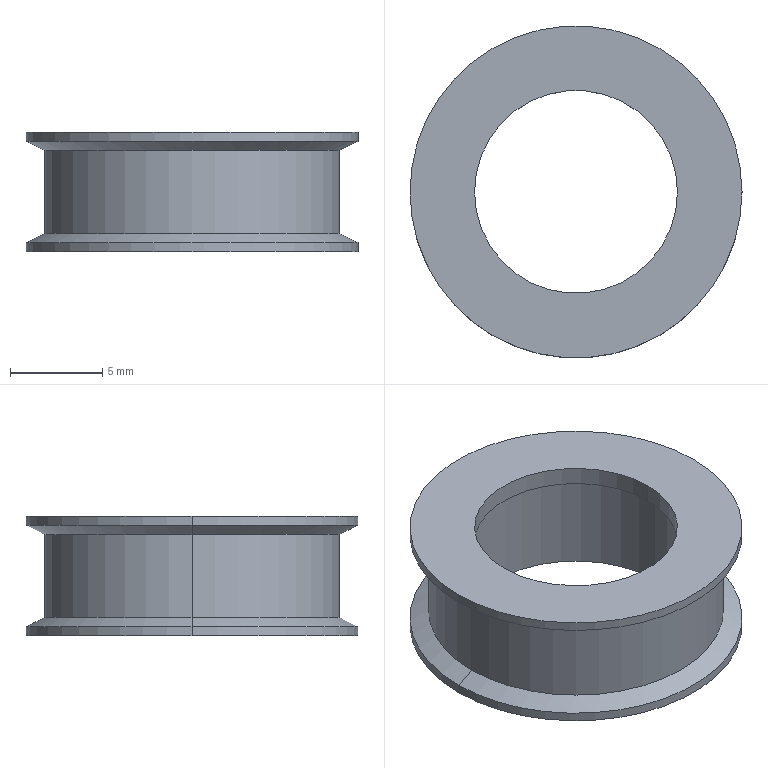Part | STEP file | 602-08-0005 | 1 solid | 17 faces | box 18 x 18 x 6.5 mm | volume 669.421 mm3 | cylinder 10 | cone 4 | plane 3 | commonest cylinder face diameters 18 x4 11 x2 12 x2 16 x2
STEP:
#1=CARTESIAN_POINT('',(0.,0.,0.));
#2=DIRECTION('',(0.,0.,1.));
#3=DIRECTION('',(1.,0.,0.));
#4=AXIS2_PLACEMENT_3D('',#1,#2,#3);
#5=CARTESIAN_POINT('',(-6.,0.,5.5));
#6=VERTEX_POINT('',#5);
#7=CARTESIAN_POINT('',(-6.,0.,0.));
#8=VERTEX_POINT('',#7);
#9=CARTESIAN_POINT('',(-6.,0.,5.5));
#10=DIRECTION('',(0.,0.,-1.));
#11=VECTOR('',#10,1.);
#12=LINE('',#9,#11);
#13=CARTESIAN_POINT('',(0.,0.,5.5));
#14=DIRECTION('',(0.,0.,-1.));
#15=DIRECTION('',(-1.,0.,0.));
#16=AXIS2_PLACEMENT_3D('',#13,#14,#15);
#17=CYLINDRICAL_SURFACE('',#16,6.);
#18=CARTESIAN_POINT('',(6.283,0.));
#19=DIRECTION('',(0.,1.));
#20=VECTOR('',#19,1.);
#21=LINE('',#18,#20);
#22=(GEOMETRIC_REPRESENTATION_CONTEXT(2)PARAMETRIC_REPRESENTATION_CONTEXT()REPRESENTATION_CONTEXT('',''));
#23=DEFINITIONAL_REPRESENTATION('',(#21),#22);
#24=PCURVE('',#17,#23);
#25=CARTESIAN_POINT('',(0.,0.,5.5));
#26=DIRECTION('',(0.,0.,-1.));
#27=DIRECTION('',(-1.,0.,0.));
#28=AXIS2_PLACEMENT_3D('',#25,#26,#27);
#29=CYLINDRICAL_SURFACE('',#28,6.);
#30=CARTESIAN_POINT('',(0.,0.));
#31=DIRECTION('',(0.,1.));
#32=VECTOR('',#31,1.);
#33=LINE('',#30,#32);
#34=(GEOMETRIC_REPRESENTATION_CONTEXT(2)PARAMETRIC_REPRESENTATION_CONTEXT()REPRESENTATION_CONTEXT('',''));
#35=DEFINITIONAL_REPRESENTATION('',(#33),#34);
#36=PCURVE('',#29,#35);
#37=SURFACE_CURVE('',#12,(#24,#36),.PCURVE_S1.);
#38=EDGE_CURVE('',#6,#8,#37,.T.);
#39=ORIENTED_EDGE('',*,*,#38,.T.);
#40=CARTESIAN_POINT('',(6.,0.,0.));
#41=VERTEX_POINT('',#40);
#42=CARTESIAN_POINT('',(0.,0.,0.));
#43=DIRECTION('',(0.,0.,-1.));
#44=DIRECTION('',(-1.,0.,0.));
#45=AXIS2_PLACEMENT_3D('',#42,#43,#44);
#46=CIRCLE('',#45,6.);
#47=CARTESIAN_POINT('',(0.,5.5));
#48=DIRECTION('',(1.,0.));
#49=VECTOR('',#48,1.);
#50=LINE('',#47,#49);
#51=(GEOMETRIC_REPRESENTATION_CONTEXT(2)PARAMETRIC_REPRESENTATION_CONTEXT()REPRESENTATION_CONTEXT('',''));
#52=DEFINITIONAL_REPRESENTATION('',(#50),#51);
#53=PCURVE('',#17,#52);
#54=CARTESIAN_POINT('',(0.,0.,0.));
#55=DIRECTION('',(0.,0.,1.));
#56=DIRECTION('',(1.,0.,0.));
#57=AXIS2_PLACEMENT_3D('',#54,#55,#56);
#58=PLANE('',#57);
#59=CARTESIAN_POINT('',(-6.,0.));
#60=CARTESIAN_POINT('',(-6.,10.392));
#61=CARTESIAN_POINT('',(3.,5.196));
#62=CARTESIAN_POINT('',(12.,0.));
#63=CARTESIAN_POINT('',(3.,-5.196));
#64=CARTESIAN_POINT('',(-6.,-10.392));
#65=CARTESIAN_POINT('',(-6.,0.));
#66=(BOUNDED_CURVE()B_SPLINE_CURVE(2,(#59,#60,#61,#62,#63,#64,#65),.UNSPECIFIED.,.T.,.F.)B_SPLINE_CURVE_WITH_KNOTS((1,2,2,2,2,1),(-2.094,0.,2.094,4.189,6.283,8.378),.UNSPECIFIED.)CURVE()GEOMETRIC_REPRESENTATION_ITEM()RATIONAL_B_SPLINE_CURVE((1.,0.5,1.,0.5,1.,0.5,1.))REPRESENTATION_ITEM(''));
#67=(GEOMETRIC_REPRESENTATION_CONTEXT(2)PARAMETRIC_REPRESENTATION_CONTEXT()REPRESENTATION_CONTEXT('',''));
#68=DEFINITIONAL_REPRESENTATION('',(#66),#67);
#69=PCURVE('',#58,#68);
#70=SURFACE_CURVE('',#46,(#53,#69),.PCURVE_S1.);
#71=EDGE_CURVE('',#41,#8,#70,.T.);
#72=ORIENTED_EDGE('',*,*,#71,.F.);
#73=CARTESIAN_POINT('',(6.,0.,5.5));
#74=VERTEX_POINT('',#73);
#75=CARTESIAN_POINT('',(6.,0.,5.5));
#76=DIRECTION('',(0.,0.,-1.));
#77=VECTOR('',#76,1.);
#78=LINE('',#75,#77);
#79=CARTESIAN_POINT('',(3.142,0.));
#80=DIRECTION('',(0.,1.));
#81=VECTOR('',#80,1.);
#82=LINE('',#79,#81);
#83=(GEOMETRIC_REPRESENTATION_CONTEXT(2)PARAMETRIC_REPRESENTATION_CONTEXT()REPRESENTATION_CONTEXT('',''));
#84=DEFINITIONAL_REPRESENTATION('',(#82),#83);
#85=PCURVE('',#17,#84);
#86=CARTESIAN_POINT('',(3.142,0.));
#87=DIRECTION('',(0.,1.));
#88=VECTOR('',#87,1.);
#89=LINE('',#86,#88);
#90=(GEOMETRIC_REPRESENTATION_CONTEXT(2)PARAMETRIC_REPRESENTATION_CONTEXT()REPRESENTATION_CONTEXT('',''));
#91=DEFINITIONAL_REPRESENTATION('',(#89),#90);
#92=PCURVE('',#29,#91);
#93=SURFACE_CURVE('',#78,(#85,#92),.PCURVE_S1.);
#94=EDGE_CURVE('',#74,#41,#93,.T.);
#95=ORIENTED_EDGE('',*,*,#94,.F.);
#96=CARTESIAN_POINT('',(0.,0.,5.5));
#97=DIRECTION('',(0.,0.,-1.));
#98=DIRECTION('',(-1.,0.,0.));
#99=AXIS2_PLACEMENT_3D('',#96,#97,#98);
#100=CIRCLE('',#99,6.);
#101=CARTESIAN_POINT('',(0.,0.));
#102=DIRECTION('',(1.,0.));
#103=VECTOR('',#102,1.);
#104=LINE('',#101,#103);
#105=(GEOMETRIC_REPRESENTATION_CONTEXT(2)PARAMETRIC_REPRESENTATION_CONTEXT()REPRESENTATION_CONTEXT('',''));
#106=DEFINITIONAL_REPRESENTATION('',(#104),#105);
#107=PCURVE('',#17,#106);
#108=CARTESIAN_POINT('',(0.,0.,5.5));
#109=DIRECTION('',(0.,0.,-1.));
#110=DIRECTION('',(-1.,0.,0.));
#111=AXIS2_PLACEMENT_3D('',#108,#109,#110);
#112=PLANE('',#111);
#113=CARTESIAN_POINT('',(0.,0.));
#114=DIRECTION('',(1.,0.));
#115=AXIS2_PLACEMENT_2D('',#113,#114);
#116=CIRCLE('',#115,6.);
#117=(GEOMETRIC_REPRESENTATION_CONTEXT(2)PARAMETRIC_REPRESENTATION_CONTEXT()REPRESENTATION_CONTEXT('',''));
#118=DEFINITIONAL_REPRESENTATION('',(#116),#117);
#119=PCURVE('',#112,#118);
#120=SURFACE_CURVE('',#100,(#107,#119),.PCURVE_S1.);
#121=EDGE_CURVE('',#74,#6,#120,.T.);
#122=ORIENTED_EDGE('',*,*,#121,.T.);
#123=EDGE_LOOP('',(#39,#72,#95,#122));
#124=FACE_BOUND('',#123,.F.);
#125=ADVANCED_FACE('',(#124),#17,.F.);
#126=CARTESIAN_POINT('',(5.5,0.,5.5));
#127=VERTEX_POINT('',#126);
#128=CARTESIAN_POINT('',(5.5,0.,6.5));
#129=VERTEX_POINT('',#128);
#130=CARTESIAN_POINT('',(5.5,0.,5.5));
#131=DIRECTION('',(0.,0.,1.));
#132=VECTOR('',#131,1.);
#133=LINE('',#130,#132);
#134=CARTESIAN_POINT('',(0.,0.,5.5));
#135=DIRECTION('',(0.,0.,1.));
#136=DIRECTION('',(1.,0.,0.));
#137=AXIS2_PLACEMENT_3D('',#134,#135,#136);
#138=CYLINDRICAL_SURFACE('',#137,5.5);
#139=CARTESIAN_POINT('',(6.283,0.));
#140=DIRECTION('',(0.,1.));
#141=VECTOR('',#140,1.);
#142=LINE('',#139,#141);
#143=(GEOMETRIC_REPRESENTATION_CONTEXT(2)PARAMETRIC_REPRESENTATION_CONTEXT()REPRESENTATION_CONTEXT('',''));
#144=DEFINITIONAL_REPRESENTATION('',(#142),#143);
#145=PCURVE('',#138,#144);
#146=CARTESIAN_POINT('',(0.,0.,5.5));
#147=DIRECTION('',(0.,0.,1.));
#148=DIRECTION('',(1.,0.,0.));
#149=AXIS2_PLACEMENT_3D('',#146,#147,#148);
#150=CYLINDRICAL_SURFACE('',#149,5.5);
#151=CARTESIAN_POINT('',(0.,0.));
#152=DIRECTION('',(0.,1.));
#153=VECTOR('',#152,1.);
#154=LINE('',#151,#153);
#155=(GEOMETRIC_REPRESENTATION_CONTEXT(2)PARAMETRIC_REPRESENTATION_CONTEXT()REPRESENTATION_CONTEXT('',''));
#156=DEFINITIONAL_REPRESENTATION('',(#154),#155);
#157=PCURVE('',#150,#156);
#158=SURFACE_CURVE('',#133,(#145,#157),.PCURVE_S1.);
#159=EDGE_CURVE('',#127,#129,#158,.T.);
#160=ORIENTED_EDGE('',*,*,#159,.T.);
#161=CARTESIAN_POINT('',(-5.5,0.,6.5));
#162=VERTEX_POINT('',#161);
#163=CARTESIAN_POINT('',(0.,0.,6.5));
#164=DIRECTION('',(0.,0.,1.));
#165=DIRECTION('',(1.,0.,0.));
#166=AXIS2_PLACEMENT_3D('',#163,#164,#165);
#167=CIRCLE('',#166,5.5);
#168=CARTESIAN_POINT('',(0.,1.));
#169=DIRECTION('',(1.,0.));
#170=VECTOR('',#169,1.);
#171=LINE('',#168,#170);
#172=(GEOMETRIC_REPRESENTATION_CONTEXT(2)PARAMETRIC_REPRESENTATION_CONTEXT()REPRESENTATION_CONTEXT('',''));
#173=DEFINITIONAL_REPRESENTATION('',(#171),#172);
#174=PCURVE('',#138,#173);
#175=CARTESIAN_POINT('',(0.,0.,6.5));
#176=DIRECTION('',(0.,0.,1.));
#177=DIRECTION('',(1.,0.,0.));
#178=AXIS2_PLACEMENT_3D('',#175,#176,#177);
#179=PLANE('',#178);
#180=CARTESIAN_POINT('',(0.,0.));
#181=DIRECTION('',(1.,0.));
#182=AXIS2_PLACEMENT_2D('',#180,#181);
#183=CIRCLE('',#182,5.5);
#184=(GEOMETRIC_REPRESENTATION_CONTEXT(2)PARAMETRIC_REPRESENTATION_CONTEXT()REPRESENTATION_CONTEXT('',''));
#185=DEFINITIONAL_REPRESENTATION('',(#183),#184);
#186=PCURVE('',#179,#185);
#187=SURFACE_CURVE('',#167,(#174,#186),.PCURVE_S1.);
#188=EDGE_CURVE('',#162,#129,#187,.T.);
#189=ORIENTED_EDGE('',*,*,#188,.F.);
#190=CARTESIAN_POINT('',(-5.5,0.,5.5));
#191=VERTEX_POINT('',#190);
#192=CARTESIAN_POINT('',(-5.5,0.,5.5));
#193=DIRECTION('',(0.,0.,1.));
#194=VECTOR('',#193,1.);
#195=LINE('',#192,#194);
#196=CARTESIAN_POINT('',(3.142,0.));
#197=DIRECTION('',(0.,1.));
#198=VECTOR('',#197,1.);
#199=LINE('',#196,#198);
#200=(GEOMETRIC_REPRESENTATION_CONTEXT(2)PARAMETRIC_REPRESENTATION_CONTEXT()REPRESENTATION_CONTEXT('',''));
#201=DEFINITIONAL_REPRESENTATION('',(#199),#200);
#202=PCURVE('',#138,#201);
#203=CARTESIAN_POINT('',(3.142,0.));
#204=DIRECTION('',(0.,1.));
#205=VECTOR('',#204,1.);
#206=LINE('',#203,#205);
#207=(GEOMETRIC_REPRESENTATION_CONTEXT(2)PARAMETRIC_REPRESENTATION_CONTEXT()REPRESENTATION_CONTEXT('',''));
#208=DEFINITIONAL_REPRESENTATION('',(#206),#207);
#209=PCURVE('',#150,#208);
#210=SURFACE_CURVE('',#195,(#202,#209),.PCURVE_S1.);
#211=EDGE_CURVE('',#191,#162,#210,.T.);
#212=ORIENTED_EDGE('',*,*,#211,.F.);
#213=CARTESIAN_POINT('',(0.,0.,5.5));
#214=DIRECTION('',(0.,0.,1.));
#215=DIRECTION('',(-1.,0.,0.));
#216=AXIS2_PLACEMENT_3D('',#213,#214,#215);
#217=CIRCLE('',#216,5.5);
#218=CARTESIAN_POINT('',(3.142,0.));
#219=DIRECTION('',(1.,0.));
#220=VECTOR('',#219,1.);
#221=LINE('',#218,#220);
#222=(GEOMETRIC_REPRESENTATION_CONTEXT(2)PARAMETRIC_REPRESENTATION_CONTEXT()REPRESENTATION_CONTEXT('',''));
#223=DEFINITIONAL_REPRESENTATION('',(#221),#222);
#224=PCURVE('',#138,#223);
#225=CARTESIAN_POINT('',(5.5,0.));
#226=CARTESIAN_POINT('',(5.5,-9.526));
#227=CARTESIAN_POINT('',(-2.75,-4.763));
#228=CARTESIAN_POINT('',(-11.,0.));
#229=CARTESIAN_POINT('',(-2.75,4.763));
#230=CARTESIAN_POINT('',(5.5,9.526));
#231=CARTESIAN_POINT('',(5.5,0.));
#232=(BOUNDED_CURVE()B_SPLINE_CURVE(2,(#225,#226,#227,#228,#229,#230,#231),.UNSPECIFIED.,.T.,.F.)B_SPLINE_CURVE_WITH_KNOTS((1,2,2,2,2,1),(-2.094,0.,2.094,4.189,6.283,8.378),.UNSPECIFIED.)CURVE()GEOMETRIC_REPRESENTATION_ITEM()RATIONAL_B_SPLINE_CURVE((1.,0.5,1.,0.5,1.,0.5,1.))REPRESENTATION_ITEM(''));
#233=(GEOMETRIC_REPRESENTATION_CONTEXT(2)PARAMETRIC_REPRESENTATION_CONTEXT()REPRESENTATION_CONTEXT('',''));
#234=DEFINITIONAL_REPRESENTATION('',(#232),#233);
#235=PCURVE('',#112,#234);
#236=SURFACE_CURVE('',#217,(#224,#235),.PCURVE_S1.);
#237=EDGE_CURVE('',#191,#127,#236,.T.);
#238=ORIENTED_EDGE('',*,*,#237,.T.);
#239=EDGE_LOOP('',(#160,#189,#212,#238));
#240=FACE_BOUND('',#239,.F.);
#241=ADVANCED_FACE('',(#240),#138,.F.);
#242=CARTESIAN_POINT('',(8.,0.,5.5));
#243=VERTEX_POINT('',#242);
#244=CARTESIAN_POINT('',(-8.,0.,5.5));
#245=VERTEX_POINT('',#244);
#246=CARTESIAN_POINT('',(0.,0.,5.5));
#247=DIRECTION('',(0.,0.,1.));
#248=DIRECTION('',(1.,0.,0.));
#249=AXIS2_PLACEMENT_3D('',#246,#247,#248);
#250=CIRCLE('',#249,8.);
#251=CARTESIAN_POINT('',(0.,0.,6.));
#252=DIRECTION('',(0.,0.,1.));
#253=DIRECTION('',(1.,0.,0.));
#254=AXIS2_PLACEMENT_3D('',#251,#252,#253);
#255=CONICAL_SURFACE('',#254,9.,1.107);
#256=CARTESIAN_POINT('',(0.,-0.5));
#257=DIRECTION('',(1.,0.));
#258=VECTOR('',#257,1.);
#259=LINE('',#256,#258);
#260=(GEOMETRIC_REPRESENTATION_CONTEXT(2)PARAMETRIC_REPRESENTATION_CONTEXT()REPRESENTATION_CONTEXT('',''));
#261=DEFINITIONAL_REPRESENTATION('',(#259),#260);
#262=PCURVE('',#255,#261);
#263=CARTESIAN_POINT('',(0.,0.,5.5));
#264=DIRECTION('',(0.,0.,-1.));
#265=DIRECTION('',(-1.,0.,0.));
#266=AXIS2_PLACEMENT_3D('',#263,#264,#265);
#267=CYLINDRICAL_SURFACE('',#266,8.);
#268=CARTESIAN_POINT('',(3.142,0.));
#269=DIRECTION('',(-1.,0.));
#270=VECTOR('',#269,1.);
#271=LINE('',#268,#270);
#272=(GEOMETRIC_REPRESENTATION_CONTEXT(2)PARAMETRIC_REPRESENTATION_CONTEXT()REPRESENTATION_CONTEXT('',''));
#273=DEFINITIONAL_REPRESENTATION('',(#271),#272);
#274=PCURVE('',#267,#273);
#275=SURFACE_CURVE('',#250,(#262,#274),.PCURVE_S1.);
#276=EDGE_CURVE('',#243,#245,#275,.T.);
#277=ORIENTED_EDGE('',*,*,#276,.T.);
#278=CARTESIAN_POINT('',(-9.,0.,6.));
#279=VERTEX_POINT('',#278);
#280=CARTESIAN_POINT('',(-9.,0.,6.));
#281=DIRECTION('',(-0.8944,0.,0.4472));
#282=VECTOR('',#281,1.);
#283=LINE('',#280,#282);
#284=CARTESIAN_POINT('',(3.142,0.));
#285=DIRECTION('',(0.,1.));
#286=VECTOR('',#285,1.);
#287=LINE('',#284,#286);
#288=(GEOMETRIC_REPRESENTATION_CONTEXT(2)PARAMETRIC_REPRESENTATION_CONTEXT()REPRESENTATION_CONTEXT('',''));
#289=DEFINITIONAL_REPRESENTATION('',(#287),#288);
#290=PCURVE('',#255,#289);
#291=CARTESIAN_POINT('',(0.,0.,6.));
#292=DIRECTION('',(0.,0.,1.));
#293=DIRECTION('',(1.,0.,0.));
#294=AXIS2_PLACEMENT_3D('',#291,#292,#293);
#295=CONICAL_SURFACE('',#294,9.,1.107);
#296=CARTESIAN_POINT('',(3.142,0.));
#297=DIRECTION('',(0.,1.));
#298=VECTOR('',#297,1.);
#299=LINE('',#296,#298);
#300=(GEOMETRIC_REPRESENTATION_CONTEXT(2)PARAMETRIC_REPRESENTATION_CONTEXT()REPRESENTATION_CONTEXT('',''));
#301=DEFINITIONAL_REPRESENTATION('',(#299),#300);
#302=PCURVE('',#295,#301);
#303=SURFACE_CURVE('',#283,(#290,#302),.PCURVE_S1.);
#304=EDGE_CURVE('',#245,#279,#303,.T.);
#305=ORIENTED_EDGE('',*,*,#304,.T.);
#306=CARTESIAN_POINT('',(9.,0.,6.));
#307=VERTEX_POINT('',#306);
#308=CARTESIAN_POINT('',(0.,0.,6.));
#309=DIRECTION('',(0.,0.,1.));
#310=DIRECTION('',(1.,0.,0.));
#311=AXIS2_PLACEMENT_3D('',#308,#309,#310);
#312=CIRCLE('',#311,9.);
#313=CARTESIAN_POINT('',(0.,0.));
#314=DIRECTION('',(1.,0.));
#315=VECTOR('',#314,1.);
#316=LINE('',#313,#315);
#317=(GEOMETRIC_REPRESENTATION_CONTEXT(2)PARAMETRIC_REPRESENTATION_CONTEXT()REPRESENTATION_CONTEXT('',''));
#318=DEFINITIONAL_REPRESENTATION('',(#316),#317);
#319=PCURVE('',#255,#318);
#320=CARTESIAN_POINT('',(0.,0.,6.5));
#321=DIRECTION('',(0.,0.,-1.));
#322=DIRECTION('',(-1.,0.,0.));
#323=AXIS2_PLACEMENT_3D('',#320,#321,#322);
#324=CYLINDRICAL_SURFACE('',#323,9.);
#325=CARTESIAN_POINT('',(3.142,0.5));
#326=DIRECTION('',(-1.,0.));
#327=VECTOR('',#326,1.);
#328=LINE('',#325,#327);
#329=(GEOMETRIC_REPRESENTATION_CONTEXT(2)PARAMETRIC_REPRESENTATION_CONTEXT()REPRESENTATION_CONTEXT('',''));
#330=DEFINITIONAL_REPRESENTATION('',(#328),#329);
#331=PCURVE('',#324,#330);
#332=SURFACE_CURVE('',#312,(#319,#331),.PCURVE_S1.);
#333=EDGE_CURVE('',#307,#279,#332,.T.);
#334=ORIENTED_EDGE('',*,*,#333,.F.);
#335=CARTESIAN_POINT('',(9.,0.,6.));
#336=DIRECTION('',(0.8944,0.,0.4472));
#337=VECTOR('',#336,1.);
#338=LINE('',#335,#337);
#339=CARTESIAN_POINT('',(0.,0.));
#340=DIRECTION('',(0.,1.));
#341=VECTOR('',#340,1.);
#342=LINE('',#339,#341);
#343=(GEOMETRIC_REPRESENTATION_CONTEXT(2)PARAMETRIC_REPRESENTATION_CONTEXT()REPRESENTATION_CONTEXT('',''));
#344=DEFINITIONAL_REPRESENTATION('',(#342),#343);
#345=PCURVE('',#255,#344);
#346=CARTESIAN_POINT('',(6.283,0.));
#347=DIRECTION('',(0.,1.));
#348=VECTOR('',#347,1.);
#349=LINE('',#346,#348);
#350=(GEOMETRIC_REPRESENTATION_CONTEXT(2)PARAMETRIC_REPRESENTATION_CONTEXT()REPRESENTATION_CONTEXT('',''));
#351=DEFINITIONAL_REPRESENTATION('',(#349),#350);
#352=PCURVE('',#295,#351);
#353=SURFACE_CURVE('',#338,(#345,#352),.PCURVE_S1.);
#354=EDGE_CURVE('',#243,#307,#353,.T.);
#355=ORIENTED_EDGE('',*,*,#354,.F.);
#356=EDGE_LOOP('',(#277,#305,#334,#355));
#357=FACE_BOUND('',#356,.T.);
#358=ADVANCED_FACE('',(#357),#255,.T.);
#359=CARTESIAN_POINT('',(8.,0.,1.));
#360=VERTEX_POINT('',#359);
#361=CARTESIAN_POINT('',(-8.,0.,1.));
#362=VERTEX_POINT('',#361);
#363=CARTESIAN_POINT('',(0.,0.,1.));
#364=DIRECTION('',(0.,0.,1.));
#365=DIRECTION('',(1.,0.,0.));
#366=AXIS2_PLACEMENT_3D('',#363,#364,#365);
#367=CIRCLE('',#366,8.);
#368=CARTESIAN_POINT('',(0.,0.,1.));
#369=DIRECTION('',(0.,0.,-1.));
#370=DIRECTION('',(-1.,0.,0.));
#371=AXIS2_PLACEMENT_3D('',#368,#369,#370);
#372=CONICAL_SURFACE('',#371,8.,1.107);
#373=CARTESIAN_POINT('',(3.142,0.));
#374=DIRECTION('',(-1.,0.));
#375=VECTOR('',#374,1.);
#376=LINE('',#373,#375);
#377=(GEOMETRIC_REPRESENTATION_CONTEXT(2)PARAMETRIC_REPRESENTATION_CONTEXT()REPRESENTATION_CONTEXT('',''));
#378=DEFINITIONAL_REPRESENTATION('',(#376),#377);
#379=PCURVE('',#372,#378);
#380=CARTESIAN_POINT('',(3.142,4.5));
#381=DIRECTION('',(-1.,0.));
#382=VECTOR('',#381,1.);
#383=LINE('',#380,#382);
#384=(GEOMETRIC_REPRESENTATION_CONTEXT(2)PARAMETRIC_REPRESENTATION_CONTEXT()REPRESENTATION_CONTEXT('',''));
#385=DEFINITIONAL_REPRESENTATION('',(#383),#384);
#386=PCURVE('',#267,#385);
#387=SURFACE_CURVE('',#367,(#379,#386),.PCURVE_S1.);
#388=EDGE_CURVE('',#360,#362,#387,.T.);
#389=ORIENTED_EDGE('',*,*,#388,.F.);
#390=CARTESIAN_POINT('',(9.,0.,0.5));
#391=VERTEX_POINT('',#390);
#392=CARTESIAN_POINT('',(8.,0.,1.));
#393=DIRECTION('',(0.8944,0.,-0.4472));
#394=VECTOR('',#393,1.);
#395=LINE('',#392,#394);
#396=CARTESIAN_POINT('',(3.142,0.));
#397=DIRECTION('',(0.,1.));
#398=VECTOR('',#397,1.);
#399=LINE('',#396,#398);
#400=(GEOMETRIC_REPRESENTATION_CONTEXT(2)PARAMETRIC_REPRESENTATION_CONTEXT()REPRESENTATION_CONTEXT('',''));
#401=DEFINITIONAL_REPRESENTATION('',(#399),#400);
#402=PCURVE('',#372,#401);
#403=CARTESIAN_POINT('',(0.,0.,1.));
#404=DIRECTION('',(0.,0.,-1.));
#405=DIRECTION('',(-1.,0.,0.));
#406=AXIS2_PLACEMENT_3D('',#403,#404,#405);
#407=CONICAL_SURFACE('',#406,8.,1.107);
#408=CARTESIAN_POINT('',(3.142,0.));
#409=DIRECTION('',(0.,1.));
#410=VECTOR('',#409,1.);
#411=LINE('',#408,#410);
#412=(GEOMETRIC_REPRESENTATION_CONTEXT(2)PARAMETRIC_REPRESENTATION_CONTEXT()REPRESENTATION_CONTEXT('',''));
#413=DEFINITIONAL_REPRESENTATION('',(#411),#412);
#414=PCURVE('',#407,#413);
#415=SURFACE_CURVE('',#395,(#402,#414),.PCURVE_S1.);
#416=EDGE_CURVE('',#360,#391,#415,.T.);
#417=ORIENTED_EDGE('',*,*,#416,.T.);
#418=CARTESIAN_POINT('',(-9.,0.,0.5));
#419=VERTEX_POINT('',#418);
#420=CARTESIAN_POINT('',(0.,0.,0.5));
#421=DIRECTION('',(0.,0.,-1.));
#422=DIRECTION('',(1.,0.,0.));
#423=AXIS2_PLACEMENT_3D('',#420,#421,#422);
#424=CIRCLE('',#423,9.);
#425=CARTESIAN_POINT('',(-3.142,0.5));
#426=DIRECTION('',(1.,0.));
#427=VECTOR('',#426,1.);
#428=LINE('',#425,#427);
#429=(GEOMETRIC_REPRESENTATION_CONTEXT(2)PARAMETRIC_REPRESENTATION_CONTEXT()REPRESENTATION_CONTEXT('',''));
#430=DEFINITIONAL_REPRESENTATION('',(#428),#429);
#431=PCURVE('',#372,#430);
#432=CARTESIAN_POINT('',(0.,0.,1.));
#433=DIRECTION('',(0.,0.,-1.));
#434=DIRECTION('',(-1.,0.,0.));
#435=AXIS2_PLACEMENT_3D('',#432,#433,#434);
#436=CYLINDRICAL_SURFACE('',#435,9.);
#437=CARTESIAN_POINT('',(-3.142,0.5));
#438=DIRECTION('',(1.,0.));
#439=VECTOR('',#438,1.);
#440=LINE('',#437,#439);
#441=(GEOMETRIC_REPRESENTATION_CONTEXT(2)PARAMETRIC_REPRESENTATION_CONTEXT()REPRESENTATION_CONTEXT('',''));
#442=DEFINITIONAL_REPRESENTATION('',(#440),#441);
#443=PCURVE('',#436,#442);
#444=SURFACE_CURVE('',#424,(#431,#443),.PCURVE_S1.);
#445=EDGE_CURVE('',#419,#391,#444,.T.);
#446=ORIENTED_EDGE('',*,*,#445,.F.);
#447=CARTESIAN_POINT('',(-8.,0.,1.));
#448=DIRECTION('',(-0.8944,0.,-0.4472));
#449=VECTOR('',#448,1.);
#450=LINE('',#447,#449);
#451=CARTESIAN_POINT('',(0.,0.));
#452=DIRECTION('',(0.,1.));
#453=VECTOR('',#452,1.);
#454=LINE('',#451,#453);
#455=(GEOMETRIC_REPRESENTATION_CONTEXT(2)PARAMETRIC_REPRESENTATION_CONTEXT()REPRESENTATION_CONTEXT('',''));
#456=DEFINITIONAL_REPRESENTATION('',(#454),#455);
#457=PCURVE('',#372,#456);
#458=CARTESIAN_POINT('',(6.283,0.));
#459=DIRECTION('',(0.,1.));
#460=VECTOR('',#459,1.);
#461=LINE('',#458,#460);
#462=(GEOMETRIC_REPRESENTATION_CONTEXT(2)PARAMETRIC_REPRESENTATION_CONTEXT()REPRESENTATION_CONTEXT('',''));
#463=DEFINITIONAL_REPRESENTATION('',(#461),#462);
#464=PCURVE('',#407,#463);
#465=SURFACE_CURVE('',#450,(#457,#464),.PCURVE_S1.);
#466=EDGE_CURVE('',#362,#419,#465,.T.);
#467=ORIENTED_EDGE('',*,*,#466,.F.);
#468=EDGE_LOOP('',(#389,#417,#446,#467));
#469=FACE_BOUND('',#468,.T.);
#470=ADVANCED_FACE('',(#469),#372,.T.);
#471=CARTESIAN_POINT('',(9.,0.,6.5));
#472=VERTEX_POINT('',#471);
#473=CARTESIAN_POINT('',(-9.,0.,6.5));
#474=VERTEX_POINT('',#473);
#475=CARTESIAN_POINT('',(0.,0.,6.5));
#476=DIRECTION('',(0.,0.,1.));
#477=DIRECTION('',(1.,0.,0.));
#478=AXIS2_PLACEMENT_3D('',#475,#476,#477);
#479=CIRCLE('',#478,9.);
#480=CARTESIAN_POINT('',(3.142,0.));
#481=DIRECTION('',(-1.,0.));
#482=VECTOR('',#481,1.);
#483=LINE('',#480,#482);
#484=(GEOMETRIC_REPRESENTATION_CONTEXT(2)PARAMETRIC_REPRESENTATION_CONTEXT()REPRESENTATION_CONTEXT('',''));
#485=DEFINITIONAL_REPRESENTATION('',(#483),#484);
#486=PCURVE('',#324,#485);
#487=CARTESIAN_POINT('',(0.,0.));
#488=DIRECTION('',(1.,0.));
#489=AXIS2_PLACEMENT_2D('',#487,#488);
#490=CIRCLE('',#489,9.);
#491=(GEOMETRIC_REPRESENTATION_CONTEXT(2)PARAMETRIC_REPRESENTATION_CONTEXT()REPRESENTATION_CONTEXT('',''));
#492=DEFINITIONAL_REPRESENTATION('',(#490),#491);
#493=PCURVE('',#179,#492);
#494=SURFACE_CURVE('',#479,(#486,#493),.PCURVE_S1.);
#495=EDGE_CURVE('',#472,#474,#494,.T.);
#496=ORIENTED_EDGE('',*,*,#495,.F.);
#497=CARTESIAN_POINT('',(9.,0.,6.5));
#498=DIRECTION('',(0.,0.,-1.));
#499=VECTOR('',#498,1.);
#500=LINE('',#497,#499);
#501=CARTESIAN_POINT('',(3.142,0.));
#502=DIRECTION('',(0.,1.));
#503=VECTOR('',#502,1.);
#504=LINE('',#501,#503);
#505=(GEOMETRIC_REPRESENTATION_CONTEXT(2)PARAMETRIC_REPRESENTATION_CONTEXT()REPRESENTATION_CONTEXT('',''));
#506=DEFINITIONAL_REPRESENTATION('',(#504),#505);
#507=PCURVE('',#324,#506);
#508=CARTESIAN_POINT('',(0.,0.,6.5));
#509=DIRECTION('',(0.,0.,-1.));
#510=DIRECTION('',(-1.,0.,0.));
#511=AXIS2_PLACEMENT_3D('',#508,#509,#510);
#512=CYLINDRICAL_SURFACE('',#511,9.);
#513=CARTESIAN_POINT('',(3.142,0.));
#514=DIRECTION('',(0.,1.));
#515=VECTOR('',#514,1.);
#516=LINE('',#513,#515);
#517=(GEOMETRIC_REPRESENTATION_CONTEXT(2)PARAMETRIC_REPRESENTATION_CONTEXT()REPRESENTATION_CONTEXT('',''));
#518=DEFINITIONAL_REPRESENTATION('',(#516),#517);
#519=PCURVE('',#512,#518);
#520=SURFACE_CURVE('',#500,(#507,#519),.PCURVE_S1.);
#521=EDGE_CURVE('',#472,#307,#520,.T.);
#522=ORIENTED_EDGE('',*,*,#521,.T.);
#523=ORIENTED_EDGE('',*,*,#333,.T.);
#524=CARTESIAN_POINT('',(-9.,0.,6.5));
#525=DIRECTION('',(0.,0.,-1.));
#526=VECTOR('',#525,1.);
#527=LINE('',#524,#526);
#528=CARTESIAN_POINT('',(0.,0.));
#529=DIRECTION('',(0.,1.));
#530=VECTOR('',#529,1.);
#531=LINE('',#528,#530);
#532=(GEOMETRIC_REPRESENTATION_CONTEXT(2)PARAMETRIC_REPRESENTATION_CONTEXT()REPRESENTATION_CONTEXT('',''));
#533=DEFINITIONAL_REPRESENTATION('',(#531),#532);
#534=PCURVE('',#324,#533);
#535=CARTESIAN_POINT('',(6.283,0.));
#536=DIRECTION('',(0.,1.));
#537=VECTOR('',#536,1.);
#538=LINE('',#535,#537);
#539=(GEOMETRIC_REPRESENTATION_CONTEXT(2)PARAMETRIC_REPRESENTATION_CONTEXT()REPRESENTATION_CONTEXT('',''));
#540=DEFINITIONAL_REPRESENTATION('',(#538),#539);
#541=PCURVE('',#512,#540);
#542=SURFACE_CURVE('',#527,(#534,#541),.PCURVE_S1.);
#543=EDGE_CURVE('',#474,#279,#542,.T.);
#544=ORIENTED_EDGE('',*,*,#543,.F.);
#545=EDGE_LOOP('',(#496,#522,#523,#544));
#546=FACE_BOUND('',#545,.T.);
#547=ADVANCED_FACE('',(#546),#324,.T.);
#548=ORIENTED_EDGE('',*,*,#276,.F.);
#549=CARTESIAN_POINT('',(8.,0.,5.5));
#550=DIRECTION('',(0.,0.,-1.));
#551=VECTOR('',#550,1.);
#552=LINE('',#549,#551);
#553=CARTESIAN_POINT('',(3.142,0.));
#554=DIRECTION('',(0.,1.));
#555=VECTOR('',#554,1.);
#556=LINE('',#553,#555);
#557=(GEOMETRIC_REPRESENTATION_CONTEXT(2)PARAMETRIC_REPRESENTATION_CONTEXT()REPRESENTATION_CONTEXT('',''));
#558=DEFINITIONAL_REPRESENTATION('',(#556),#557);
#559=PCURVE('',#267,#558);
#560=CARTESIAN_POINT('',(0.,0.,5.5));
#561=DIRECTION('',(0.,0.,-1.));
#562=DIRECTION('',(-1.,0.,0.));
#563=AXIS2_PLACEMENT_3D('',#560,#561,#562);
#564=CYLINDRICAL_SURFACE('',#563,8.);
#565=CARTESIAN_POINT('',(3.142,0.));
#566=DIRECTION('',(0.,1.));
#567=VECTOR('',#566,1.);
#568=LINE('',#565,#567);
#569=(GEOMETRIC_REPRESENTATION_CONTEXT(2)PARAMETRIC_REPRESENTATION_CONTEXT()REPRESENTATION_CONTEXT('',''));
#570=DEFINITIONAL_REPRESENTATION('',(#568),#569);
#571=PCURVE('',#564,#570);
#572=SURFACE_CURVE('',#552,(#559,#571),.PCURVE_S1.);
#573=EDGE_CURVE('',#243,#360,#572,.T.);
#574=ORIENTED_EDGE('',*,*,#573,.T.);
#575=ORIENTED_EDGE('',*,*,#388,.T.);
#576=CARTESIAN_POINT('',(-8.,0.,5.5));
#577=DIRECTION('',(0.,0.,-1.));
#578=VECTOR('',#577,1.);
#579=LINE('',#576,#578);
#580=CARTESIAN_POINT('',(0.,0.));
#581=DIRECTION('',(0.,1.));
#582=VECTOR('',#581,1.);
#583=LINE('',#580,#582);
#584=(GEOMETRIC_REPRESENTATION_CONTEXT(2)PARAMETRIC_REPRESENTATION_CONTEXT()REPRESENTATION_CONTEXT('',''));
#585=DEFINITIONAL_REPRESENTATION('',(#583),#584);
#586=PCURVE('',#267,#585);
#587=CARTESIAN_POINT('',(6.283,0.));
#588=DIRECTION('',(0.,1.));
#589=VECTOR('',#588,1.);
#590=LINE('',#587,#589);
#591=(GEOMETRIC_REPRESENTATION_CONTEXT(2)PARAMETRIC_REPRESENTATION_CONTEXT()REPRESENTATION_CONTEXT('',''));
#592=DEFINITIONAL_REPRESENTATION('',(#590),#591);
#593=PCURVE('',#564,#592);
#594=SURFACE_CURVE('',#579,(#586,#593),.PCURVE_S1.);
#595=EDGE_CURVE('',#245,#362,#594,.T.);
#596=ORIENTED_EDGE('',*,*,#595,.F.);
#597=EDGE_LOOP('',(#548,#574,#575,#596));
#598=FACE_BOUND('',#597,.T.);
#599=ADVANCED_FACE('',(#598),#267,.T.);
#600=ORIENTED_EDGE('',*,*,#445,.T.);
#601=CARTESIAN_POINT('',(9.,0.,0.));
#602=VERTEX_POINT('',#601);
#603=CARTESIAN_POINT('',(9.,0.,1.));
#604=DIRECTION('',(0.,0.,-1.));
#605=VECTOR('',#604,1.);
#606=LINE('',#603,#605);
#607=CARTESIAN_POINT('',(3.142,0.));
#608=DIRECTION('',(0.,1.));
#609=VECTOR('',#608,1.);
#610=LINE('',#607,#609);
#611=(GEOMETRIC_REPRESENTATION_CONTEXT(2)PARAMETRIC_REPRESENTATION_CONTEXT()REPRESENTATION_CONTEXT('',''));
#612=DEFINITIONAL_REPRESENTATION('',(#610),#611);
#613=PCURVE('',#436,#612);
#614=CARTESIAN_POINT('',(0.,0.,1.));
#615=DIRECTION('',(0.,0.,-1.));
#616=DIRECTION('',(-1.,0.,0.));
#617=AXIS2_PLACEMENT_3D('',#614,#615,#616);
#618=CYLINDRICAL_SURFACE('',#617,9.);
#619=CARTESIAN_POINT('',(3.142,0.));
#620=DIRECTION('',(0.,1.));
#621=VECTOR('',#620,1.);
#622=LINE('',#619,#621);
#623=(GEOMETRIC_REPRESENTATION_CONTEXT(2)PARAMETRIC_REPRESENTATION_CONTEXT()REPRESENTATION_CONTEXT('',''));
#624=DEFINITIONAL_REPRESENTATION('',(#622),#623);
#625=PCURVE('',#618,#624);
#626=SURFACE_CURVE('',#606,(#613,#625),.PCURVE_S1.);
#627=EDGE_CURVE('',#391,#602,#626,.T.);
#628=ORIENTED_EDGE('',*,*,#627,.T.);
#629=CARTESIAN_POINT('',(-9.,0.,0.));
#630=VERTEX_POINT('',#629);
#631=CARTESIAN_POINT('',(0.,0.,0.));
#632=DIRECTION('',(0.,0.,1.));
#633=DIRECTION('',(1.,0.,0.));
#634=AXIS2_PLACEMENT_3D('',#631,#632,#633);
#635=CIRCLE('',#634,9.);
#636=CARTESIAN_POINT('',(3.142,1.));
#637=DIRECTION('',(-1.,0.));
#638=VECTOR('',#637,1.);
#639=LINE('',#636,#638);
#640=(GEOMETRIC_REPRESENTATION_CONTEXT(2)PARAMETRIC_REPRESENTATION_CONTEXT()REPRESENTATION_CONTEXT('',''));
#641=DEFINITIONAL_REPRESENTATION('',(#639),#640);
#642=PCURVE('',#436,#641);
#643=CARTESIAN_POINT('',(0.,0.));
#644=DIRECTION('',(1.,0.));
#645=AXIS2_PLACEMENT_2D('',#643,#644);
#646=CIRCLE('',#645,9.);
#647=(GEOMETRIC_REPRESENTATION_CONTEXT(2)PARAMETRIC_REPRESENTATION_CONTEXT()REPRESENTATION_CONTEXT('',''));
#648=DEFINITIONAL_REPRESENTATION('',(#646),#647);
#649=PCURVE('',#58,#648);
#650=SURFACE_CURVE('',#635,(#642,#649),.PCURVE_S1.);
#651=EDGE_CURVE('',#602,#630,#650,.T.);
#652=ORIENTED_EDGE('',*,*,#651,.T.);
#653=CARTESIAN_POINT('',(-9.,0.,1.));
#654=DIRECTION('',(0.,0.,-1.));
#655=VECTOR('',#654,1.);
#656=LINE('',#653,#655);
#657=CARTESIAN_POINT('',(0.,0.));
#658=DIRECTION('',(0.,1.));
#659=VECTOR('',#658,1.);
#660=LINE('',#657,#659);
#661=(GEOMETRIC_REPRESENTATION_CONTEXT(2)PARAMETRIC_REPRESENTATION_CONTEXT()REPRESENTATION_CONTEXT('',''));
#662=DEFINITIONAL_REPRESENTATION('',(#660),#661);
#663=PCURVE('',#436,#662);
#664=CARTESIAN_POINT('',(6.283,0.));
#665=DIRECTION('',(0.,1.));
#666=VECTOR('',#665,1.);
#667=LINE('',#664,#666);
#668=(GEOMETRIC_REPRESENTATION_CONTEXT(2)PARAMETRIC_REPRESENTATION_CONTEXT()REPRESENTATION_CONTEXT('',''));
#669=DEFINITIONAL_REPRESENTATION('',(#667),#668);
#670=PCURVE('',#618,#669);
#671=SURFACE_CURVE('',#656,(#663,#670),.PCURVE_S1.);
#672=EDGE_CURVE('',#419,#630,#671,.T.);
#673=ORIENTED_EDGE('',*,*,#672,.F.);
#674=EDGE_LOOP('',(#600,#628,#652,#673));
#675=FACE_BOUND('',#674,.T.);
#676=ADVANCED_FACE('',(#675),#436,.T.);
#677=ORIENTED_EDGE('',*,*,#627,.F.);
#678=CARTESIAN_POINT('',(0.,0.,0.5));
#679=DIRECTION('',(0.,0.,-1.));
#680=DIRECTION('',(1.,0.,0.));
#681=AXIS2_PLACEMENT_3D('',#678,#679,#680);
#682=CIRCLE('',#681,9.);
#683=CARTESIAN_POINT('',(3.142,0.5));
#684=DIRECTION('',(1.,0.));
#685=VECTOR('',#684,1.);
#686=LINE('',#683,#685);
#687=(GEOMETRIC_REPRESENTATION_CONTEXT(2)PARAMETRIC_REPRESENTATION_CONTEXT()REPRESENTATION_CONTEXT('',''));
#688=DEFINITIONAL_REPRESENTATION('',(#686),#687);
#689=PCURVE('',#618,#688);
#690=CARTESIAN_POINT('',(3.142,0.5));
#691=DIRECTION('',(1.,0.));
#692=VECTOR('',#691,1.);
#693=LINE('',#690,#692);
#694=(GEOMETRIC_REPRESENTATION_CONTEXT(2)PARAMETRIC_REPRESENTATION_CONTEXT()REPRESENTATION_CONTEXT('',''));
#695=DEFINITIONAL_REPRESENTATION('',(#693),#694);
#696=PCURVE('',#407,#695);
#697=SURFACE_CURVE('',#682,(#689,#696),.PCURVE_S1.);
#698=EDGE_CURVE('',#391,#419,#697,.T.);
#699=ORIENTED_EDGE('',*,*,#698,.T.);
#700=ORIENTED_EDGE('',*,*,#672,.T.);
#701=CARTESIAN_POINT('',(0.,0.,0.));
#702=DIRECTION('',(0.,0.,1.));
#703=DIRECTION('',(1.,0.,0.));
#704=AXIS2_PLACEMENT_3D('',#701,#702,#703);
#705=CIRCLE('',#704,9.);
#706=CARTESIAN_POINT('',(9.425,1.));
#707=DIRECTION('',(-1.,0.));
#708=VECTOR('',#707,1.);
#709=LINE('',#706,#708);
#710=(GEOMETRIC_REPRESENTATION_CONTEXT(2)PARAMETRIC_REPRESENTATION_CONTEXT()REPRESENTATION_CONTEXT('',''));
#711=DEFINITIONAL_REPRESENTATION('',(#709),#710);
#712=PCURVE('',#618,#711);
#713=CARTESIAN_POINT('',(0.,0.));
#714=DIRECTION('',(1.,0.));
#715=AXIS2_PLACEMENT_2D('',#713,#714);
#716=CIRCLE('',#715,9.);
#717=(GEOMETRIC_REPRESENTATION_CONTEXT(2)PARAMETRIC_REPRESENTATION_CONTEXT()REPRESENTATION_CONTEXT('',''));
#718=DEFINITIONAL_REPRESENTATION('',(#716),#717);
#719=PCURVE('',#58,#718);
#720=SURFACE_CURVE('',#705,(#712,#719),.PCURVE_S1.);
#721=EDGE_CURVE('',#630,#602,#720,.T.);
#722=ORIENTED_EDGE('',*,*,#721,.T.);
#723=EDGE_LOOP('',(#677,#699,#700,#722));
#724=FACE_BOUND('',#723,.T.);
#725=ADVANCED_FACE('',(#724),#618,.T.);
#726=CARTESIAN_POINT('',(0.,0.,0.));
#727=DIRECTION('',(0.,0.,-1.));
#728=DIRECTION('',(-1.,0.,0.));
#729=AXIS2_PLACEMENT_3D('',#726,#727,#728);
#730=CIRCLE('',#729,6.);
#731=CARTESIAN_POINT('',(-6.,0.));
#732=CARTESIAN_POINT('',(-6.,10.392));
#733=CARTESIAN_POINT('',(3.,5.196));
#734=CARTESIAN_POINT('',(12.,0.));
#735=CARTESIAN_POINT('',(3.,-5.196));
#736=CARTESIAN_POINT('',(-6.,-10.392));
#737=CARTESIAN_POINT('',(-6.,0.));
#738=(BOUNDED_CURVE()B_SPLINE_CURVE(2,(#731,#732,#733,#734,#735,#736,#737),.UNSPECIFIED.,.T.,.F.)B_SPLINE_CURVE_WITH_KNOTS((1,2,2,2,2,1),(-2.094,0.,2.094,4.189,6.283,8.378),.UNSPECIFIED.)CURVE()GEOMETRIC_REPRESENTATION_ITEM()RATIONAL_B_SPLINE_CURVE((1.,0.5,1.,0.5,1.,0.5,1.))REPRESENTATION_ITEM(''));
#739=(GEOMETRIC_REPRESENTATION_CONTEXT(2)PARAMETRIC_REPRESENTATION_CONTEXT()REPRESENTATION_CONTEXT('',''));
#740=DEFINITIONAL_REPRESENTATION('',(#738),#739);
#741=PCURVE('',#58,#740);
#742=CARTESIAN_POINT('',(0.,5.5));
#743=DIRECTION('',(1.,0.));
#744=VECTOR('',#743,1.);
#745=LINE('',#742,#744);
#746=(GEOMETRIC_REPRESENTATION_CONTEXT(2)PARAMETRIC_REPRESENTATION_CONTEXT()REPRESENTATION_CONTEXT('',''));
#747=DEFINITIONAL_REPRESENTATION('',(#745),#746);
#748=PCURVE('',#29,#747);
#749=SURFACE_CURVE('',#730,(#741,#748),.PCURVE_S1.);
#750=EDGE_CURVE('',#8,#41,#749,.T.);
#751=ORIENTED_EDGE('',*,*,#750,.F.);
#752=ORIENTED_EDGE('',*,*,#71,.F.);
#753=EDGE_LOOP('',(#751,#752));
#754=FACE_BOUND('',#753,.T.);
#755=ORIENTED_EDGE('',*,*,#721,.F.);
#756=ORIENTED_EDGE('',*,*,#651,.F.);
#757=EDGE_LOOP('',(#755,#756));
#758=FACE_BOUND('',#757,.T.);
#759=ADVANCED_FACE('',(#754,#758),#58,.F.);
#760=ORIENTED_EDGE('',*,*,#573,.F.);
#761=CARTESIAN_POINT('',(0.,0.,5.5));
#762=DIRECTION('',(0.,0.,1.));
#763=DIRECTION('',(1.,0.,0.));
#764=AXIS2_PLACEMENT_3D('',#761,#762,#763);
#765=CIRCLE('',#764,8.);
#766=CARTESIAN_POINT('',(9.425,0.));
#767=DIRECTION('',(-1.,0.));
#768=VECTOR('',#767,1.);
#769=LINE('',#766,#768);
#770=(GEOMETRIC_REPRESENTATION_CONTEXT(2)PARAMETRIC_REPRESENTATION_CONTEXT()REPRESENTATION_CONTEXT('',''));
#771=DEFINITIONAL_REPRESENTATION('',(#769),#770);
#772=PCURVE('',#564,#771);
#773=CARTESIAN_POINT('',(0.,-0.5));
#774=DIRECTION('',(1.,0.));
#775=VECTOR('',#774,1.);
#776=LINE('',#773,#775);
#777=(GEOMETRIC_REPRESENTATION_CONTEXT(2)PARAMETRIC_REPRESENTATION_CONTEXT()REPRESENTATION_CONTEXT('',''));
#778=DEFINITIONAL_REPRESENTATION('',(#776),#777);
#779=PCURVE('',#295,#778);
#780=SURFACE_CURVE('',#765,(#772,#779),.PCURVE_S1.);
#781=EDGE_CURVE('',#245,#243,#780,.T.);
#782=ORIENTED_EDGE('',*,*,#781,.F.);
#783=ORIENTED_EDGE('',*,*,#595,.T.);
#784=CARTESIAN_POINT('',(0.,0.,1.));
#785=DIRECTION('',(0.,0.,1.));
#786=DIRECTION('',(1.,0.,0.));
#787=AXIS2_PLACEMENT_3D('',#784,#785,#786);
#788=CIRCLE('',#787,8.);
#789=CARTESIAN_POINT('',(9.425,4.5));
#790=DIRECTION('',(-1.,0.));
#791=VECTOR('',#790,1.);
#792=LINE('',#789,#791);
#793=(GEOMETRIC_REPRESENTATION_CONTEXT(2)PARAMETRIC_REPRESENTATION_CONTEXT()REPRESENTATION_CONTEXT('',''));
#794=DEFINITIONAL_REPRESENTATION('',(#792),#793);
#795=PCURVE('',#564,#794);
#796=CARTESIAN_POINT('',(9.425,0.));
#797=DIRECTION('',(-1.,0.));
#798=VECTOR('',#797,1.);
#799=LINE('',#796,#798);
#800=(GEOMETRIC_REPRESENTATION_CONTEXT(2)PARAMETRIC_REPRESENTATION_CONTEXT()REPRESENTATION_CONTEXT('',''));
#801=DEFINITIONAL_REPRESENTATION('',(#799),#800);
#802=PCURVE('',#407,#801);
#803=SURFACE_CURVE('',#788,(#795,#802),.PCURVE_S1.);
#804=EDGE_CURVE('',#362,#360,#803,.T.);
#805=ORIENTED_EDGE('',*,*,#804,.T.);
#806=EDGE_LOOP('',(#760,#782,#783,#805));
#807=FACE_BOUND('',#806,.T.);
#808=ADVANCED_FACE('',(#807),#564,.T.);
#809=ORIENTED_EDGE('',*,*,#521,.F.);
#810=CARTESIAN_POINT('',(0.,0.,6.5));
#811=DIRECTION('',(0.,0.,1.));
#812=DIRECTION('',(1.,0.,0.));
#813=AXIS2_PLACEMENT_3D('',#810,#811,#812);
#814=CIRCLE('',#813,9.);
#815=CARTESIAN_POINT('',(9.425,0.));
#816=DIRECTION('',(-1.,0.));
#817=VECTOR('',#816,1.);
#818=LINE('',#815,#817);
#819=(GEOMETRIC_REPRESENTATION_CONTEXT(2)PARAMETRIC_REPRESENTATION_CONTEXT()REPRESENTATION_CONTEXT('',''));
#820=DEFINITIONAL_REPRESENTATION('',(#818),#819);
#821=PCURVE('',#512,#820);
#822=CARTESIAN_POINT('',(0.,0.));
#823=DIRECTION('',(1.,0.));
#824=AXIS2_PLACEMENT_2D('',#822,#823);
#825=CIRCLE('',#824,9.);
#826=(GEOMETRIC_REPRESENTATION_CONTEXT(2)PARAMETRIC_REPRESENTATION_CONTEXT()REPRESENTATION_CONTEXT('',''));
#827=DEFINITIONAL_REPRESENTATION('',(#825),#826);
#828=PCURVE('',#179,#827);
#829=SURFACE_CURVE('',#814,(#821,#828),.PCURVE_S1.);
#830=EDGE_CURVE('',#474,#472,#829,.T.);
#831=ORIENTED_EDGE('',*,*,#830,.F.);
#832=ORIENTED_EDGE('',*,*,#543,.T.);
#833=CARTESIAN_POINT('',(0.,0.,6.));
#834=DIRECTION('',(0.,0.,1.));
#835=DIRECTION('',(1.,0.,0.));
#836=AXIS2_PLACEMENT_3D('',#833,#834,#835);
#837=CIRCLE('',#836,9.);
#838=CARTESIAN_POINT('',(9.425,0.5));
#839=DIRECTION('',(-1.,0.));
#840=VECTOR('',#839,1.);
#841=LINE('',#838,#840);
#842=(GEOMETRIC_REPRESENTATION_CONTEXT(2)PARAMETRIC_REPRESENTATION_CONTEXT()REPRESENTATION_CONTEXT('',''));
#843=DEFINITIONAL_REPRESENTATION('',(#841),#842);
#844=PCURVE('',#512,#843);
#845=CARTESIAN_POINT('',(0.,0.));
#846=DIRECTION('',(1.,0.));
#847=VECTOR('',#846,1.);
#848=LINE('',#845,#847);
#849=(GEOMETRIC_REPRESENTATION_CONTEXT(2)PARAMETRIC_REPRESENTATION_CONTEXT()REPRESENTATION_CONTEXT('',''));
#850=DEFINITIONAL_REPRESENTATION('',(#848),#849);
#851=PCURVE('',#295,#850);
#852=SURFACE_CURVE('',#837,(#844,#851),.PCURVE_S1.);
#853=EDGE_CURVE('',#279,#307,#852,.T.);
#854=ORIENTED_EDGE('',*,*,#853,.T.);
#855=EDGE_LOOP('',(#809,#831,#832,#854));
#856=FACE_BOUND('',#855,.T.);
#857=ADVANCED_FACE('',(#856),#512,.T.);
#858=CARTESIAN_POINT('',(0.,0.,6.5));
#859=DIRECTION('',(0.,0.,1.));
#860=DIRECTION('',(1.,0.,0.));
#861=AXIS2_PLACEMENT_3D('',#858,#859,#860);
#862=CIRCLE('',#861,5.5);
#863=CARTESIAN_POINT('',(0.,0.));
#864=DIRECTION('',(1.,0.));
#865=AXIS2_PLACEMENT_2D('',#863,#864);
#866=CIRCLE('',#865,5.5);
#867=(GEOMETRIC_REPRESENTATION_CONTEXT(2)PARAMETRIC_REPRESENTATION_CONTEXT()REPRESENTATION_CONTEXT('',''));
#868=DEFINITIONAL_REPRESENTATION('',(#866),#867);
#869=PCURVE('',#179,#868);
#870=CARTESIAN_POINT('',(0.,1.));
#871=DIRECTION('',(1.,0.));
#872=VECTOR('',#871,1.);
#873=LINE('',#870,#872);
#874=(GEOMETRIC_REPRESENTATION_CONTEXT(2)PARAMETRIC_REPRESENTATION_CONTEXT()REPRESENTATION_CONTEXT('',''));
#875=DEFINITIONAL_REPRESENTATION('',(#873),#874);
#876=PCURVE('',#150,#875);
#877=SURFACE_CURVE('',#862,(#869,#876),.PCURVE_S1.);
#878=EDGE_CURVE('',#129,#162,#877,.T.);
#879=ORIENTED_EDGE('',*,*,#878,.F.);
#880=ORIENTED_EDGE('',*,*,#188,.F.);
#881=EDGE_LOOP('',(#879,#880));
#882=FACE_BOUND('',#881,.T.);
#883=ORIENTED_EDGE('',*,*,#830,.T.);
#884=ORIENTED_EDGE('',*,*,#495,.T.);
#885=EDGE_LOOP('',(#883,#884));
#886=FACE_BOUND('',#885,.T.);
#887=ADVANCED_FACE('',(#882,#886),#179,.T.);
#888=ORIENTED_EDGE('',*,*,#416,.F.);
#889=ORIENTED_EDGE('',*,*,#804,.F.);
#890=ORIENTED_EDGE('',*,*,#466,.T.);
#891=ORIENTED_EDGE('',*,*,#698,.F.);
#892=EDGE_LOOP('',(#888,#889,#890,#891));
#893=FACE_BOUND('',#892,.T.);
#894=ADVANCED_FACE('',(#893),#407,.T.);
#895=ORIENTED_EDGE('',*,*,#304,.F.);
#896=ORIENTED_EDGE('',*,*,#781,.T.);
#897=ORIENTED_EDGE('',*,*,#354,.T.);
#898=ORIENTED_EDGE('',*,*,#853,.F.);
#899=EDGE_LOOP('',(#895,#896,#897,#898));
#900=FACE_BOUND('',#899,.T.);
#901=ADVANCED_FACE('',(#900),#295,.T.);
#902=ORIENTED_EDGE('',*,*,#878,.F.);
#903=ORIENTED_EDGE('',*,*,#159,.F.);
#904=CARTESIAN_POINT('',(0.,0.,5.5));
#905=DIRECTION('',(0.,0.,1.));
#906=DIRECTION('',(-1.,0.,0.));
#907=AXIS2_PLACEMENT_3D('',#904,#905,#906);
#908=CIRCLE('',#907,5.5);
#909=CARTESIAN_POINT('',(-3.142,0.));
#910=DIRECTION('',(1.,0.));
#911=VECTOR('',#910,1.);
#912=LINE('',#909,#911);
#913=(GEOMETRIC_REPRESENTATION_CONTEXT(2)PARAMETRIC_REPRESENTATION_CONTEXT()REPRESENTATION_CONTEXT('',''));
#914=DEFINITIONAL_REPRESENTATION('',(#912),#913);
#915=PCURVE('',#150,#914);
#916=CARTESIAN_POINT('',(5.5,0.));
#917=CARTESIAN_POINT('',(5.5,-9.526));
#918=CARTESIAN_POINT('',(-2.75,-4.763));
#919=CARTESIAN_POINT('',(-11.,0.));
#920=CARTESIAN_POINT('',(-2.75,4.763));
#921=CARTESIAN_POINT('',(5.5,9.526));
#922=CARTESIAN_POINT('',(5.5,0.));
#923=(BOUNDED_CURVE()B_SPLINE_CURVE(2,(#916,#917,#918,#919,#920,#921,#922),.UNSPECIFIED.,.T.,.F.)B_SPLINE_CURVE_WITH_KNOTS((1,2,2,2,2,1),(-2.094,0.,2.094,4.189,6.283,8.378),.UNSPECIFIED.)CURVE()GEOMETRIC_REPRESENTATION_ITEM()RATIONAL_B_SPLINE_CURVE((1.,0.5,1.,0.5,1.,0.5,1.))REPRESENTATION_ITEM(''));
#924=(GEOMETRIC_REPRESENTATION_CONTEXT(2)PARAMETRIC_REPRESENTATION_CONTEXT()REPRESENTATION_CONTEXT('',''));
#925=DEFINITIONAL_REPRESENTATION('',(#923),#924);
#926=PCURVE('',#112,#925);
#927=SURFACE_CURVE('',#908,(#915,#926),.PCURVE_S1.);
#928=EDGE_CURVE('',#127,#191,#927,.T.);
#929=ORIENTED_EDGE('',*,*,#928,.T.);
#930=ORIENTED_EDGE('',*,*,#211,.T.);
#931=EDGE_LOOP('',(#902,#903,#929,#930));
#932=FACE_BOUND('',#931,.F.);
#933=ADVANCED_FACE('',(#932),#150,.F.);
#934=CARTESIAN_POINT('',(0.,0.,5.5));
#935=DIRECTION('',(0.,0.,-1.));
#936=DIRECTION('',(-1.,0.,0.));
#937=AXIS2_PLACEMENT_3D('',#934,#935,#936);
#938=CIRCLE('',#937,6.);
#939=CARTESIAN_POINT('',(0.,0.));
#940=DIRECTION('',(1.,0.));
#941=AXIS2_PLACEMENT_2D('',#939,#940);
#942=CIRCLE('',#941,6.);
#943=(GEOMETRIC_REPRESENTATION_CONTEXT(2)PARAMETRIC_REPRESENTATION_CONTEXT()REPRESENTATION_CONTEXT('',''));
#944=DEFINITIONAL_REPRESENTATION('',(#942),#943);
#945=PCURVE('',#112,#944);
#946=CARTESIAN_POINT('',(0.,0.));
#947=DIRECTION('',(1.,0.));
#948=VECTOR('',#947,1.);
#949=LINE('',#946,#948);
#950=(GEOMETRIC_REPRESENTATION_CONTEXT(2)PARAMETRIC_REPRESENTATION_CONTEXT()REPRESENTATION_CONTEXT('',''));
#951=DEFINITIONAL_REPRESENTATION('',(#949),#950);
#952=PCURVE('',#29,#951);
#953=SURFACE_CURVE('',#938,(#945,#952),.PCURVE_S1.);
#954=EDGE_CURVE('',#6,#74,#953,.T.);
#955=ORIENTED_EDGE('',*,*,#954,.T.);
#956=ORIENTED_EDGE('',*,*,#121,.T.);
#957=EDGE_LOOP('',(#955,#956));
#958=FACE_BOUND('',#957,.T.);
#959=ORIENTED_EDGE('',*,*,#928,.T.);
#960=ORIENTED_EDGE('',*,*,#237,.T.);
#961=EDGE_LOOP('',(#959,#960));
#962=FACE_BOUND('',#961,.T.);
#963=ADVANCED_FACE('',(#958,#962),#112,.T.);
#964=ORIENTED_EDGE('',*,*,#750,.F.);
#965=ORIENTED_EDGE('',*,*,#38,.F.);
#966=ORIENTED_EDGE('',*,*,#954,.T.);
#967=ORIENTED_EDGE('',*,*,#94,.T.);
#968=EDGE_LOOP('',(#964,#965,#966,#967));
#969=FACE_BOUND('',#968,.F.);
#970=ADVANCED_FACE('',(#969),#29,.F.);
#971=CLOSED_SHELL('',(#125,#241,#358,#470,#547,#599,#676,#725,#759,#808,#857,#887,#894,#901,#933,#963,#970));
#972=MANIFOLD_SOLID_BREP('',#971);
#973=(LENGTH_UNIT()NAMED_UNIT(*)SI_UNIT(.MILLI.,.METRE.));
#974=UNCERTAINTY_MEASURE_WITH_UNIT(LENGTH_MEASURE(0.0000001),#973,'','');
#975=(NAMED_UNIT(*)PLANE_ANGLE_UNIT()SI_UNIT($,.RADIAN.));
#976=(NAMED_UNIT(*)SI_UNIT($,.STERADIAN.)SOLID_ANGLE_UNIT());
#977=(GEOMETRIC_REPRESENTATION_CONTEXT(3)GLOBAL_UNCERTAINTY_ASSIGNED_CONTEXT((#974))GLOBAL_UNIT_ASSIGNED_CONTEXT((#973,#975,#976))REPRESENTATION_CONTEXT('',''));
#978=ADVANCED_BREP_SHAPE_REPRESENTATION('',(#4,#972),#977);